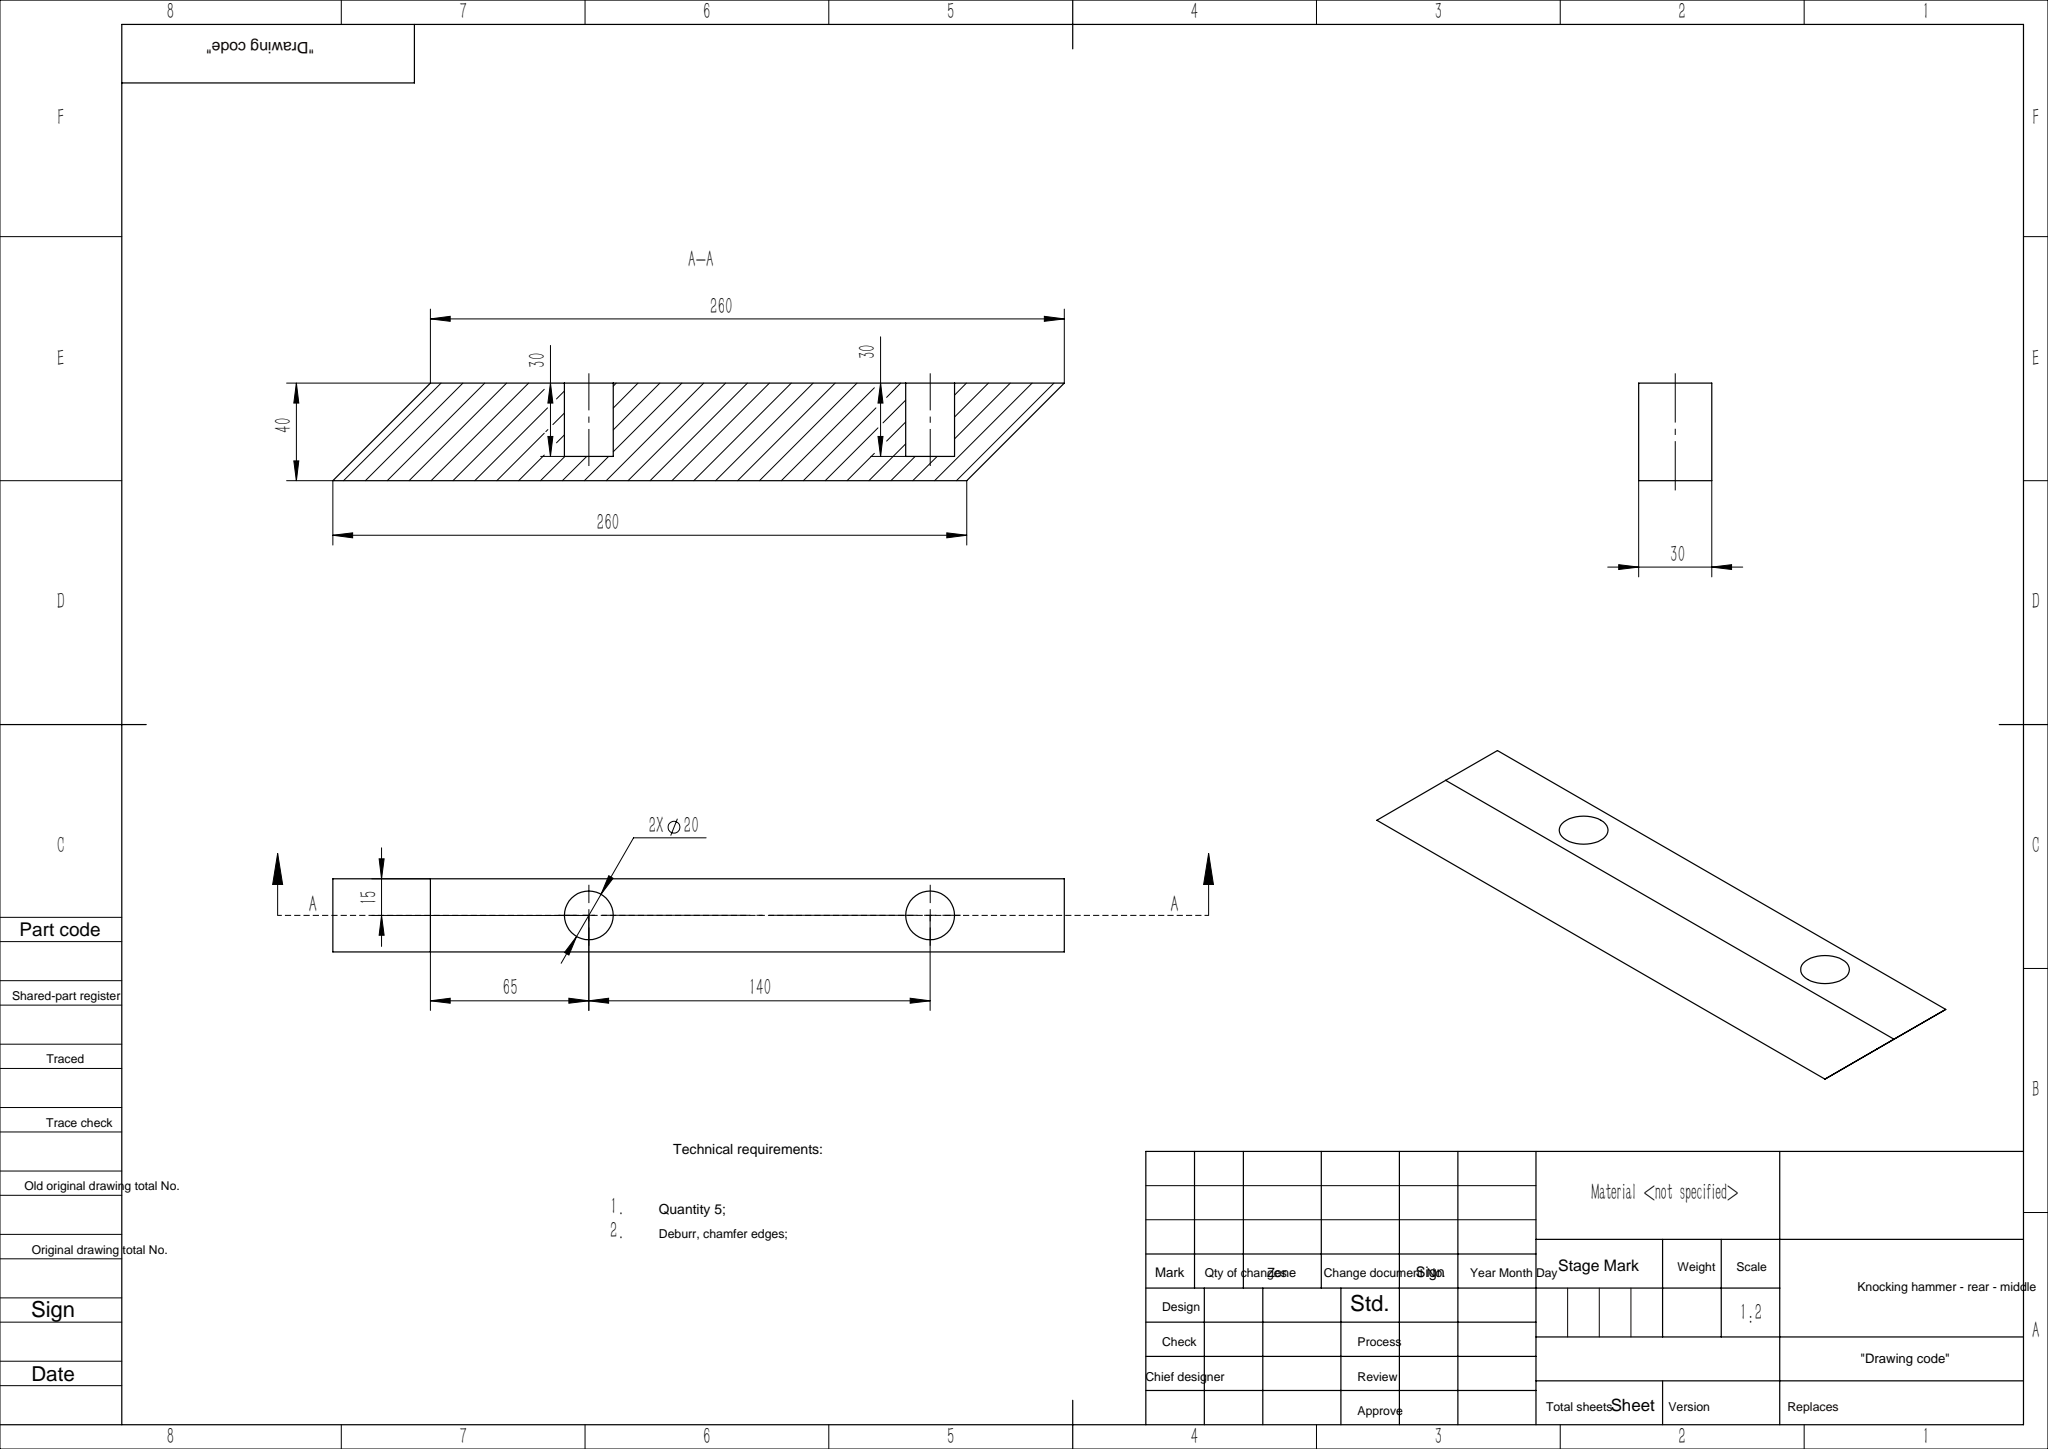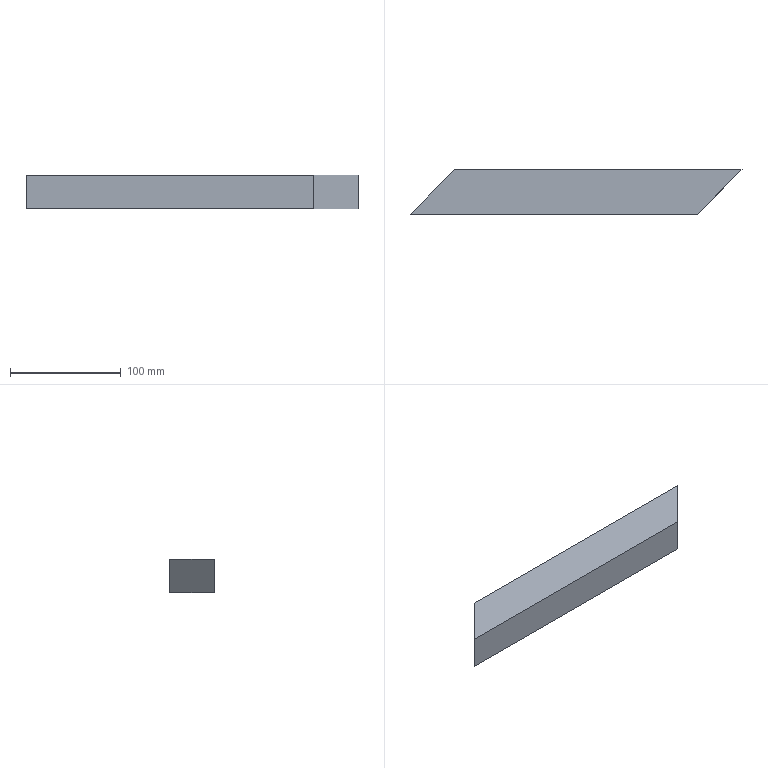Part | SolidWorks | features ICE 5, Extrusion 1 | 1 solid | 12 faces | box 300 x 40 x 30 mm | volume 293150 mm3 | plane 8 | cylinder 4 | commonest cylinder face diameters 20 x4
STEP:
#1=CARTESIAN_POINT('',(-70.,10.,-10.));
#2=VERTEX_POINT('',#1);
#3=CARTESIAN_POINT('',(-70.,10.,10.));
#4=VERTEX_POINT('',#3);
#5=CARTESIAN_POINT('',(-70.,10.,0.));
#6=DIRECTION('',(0.,1.,0.));
#7=DIRECTION('',(0.,0.,-1.));
#8=AXIS2_PLACEMENT_3D('',#5,#6,#7);
#9=CIRCLE('',#8,10.);
#10=EDGE_CURVE('',#2,#4,#9,.T.);
#11=ORIENTED_EDGE('',*,*,#10,.F.);
#12=CARTESIAN_POINT('',(-70.,40.,-10.));
#13=VERTEX_POINT('',#12);
#14=CARTESIAN_POINT('',(-70.,10.,-10.));
#15=DIRECTION('',(0.,1.,0.));
#16=VECTOR('',#15,1000.);
#17=LINE('',#14,#16);
#18=EDGE_CURVE('',#2,#13,#17,.T.);
#19=ORIENTED_EDGE('',*,*,#18,.T.);
#20=CARTESIAN_POINT('',(-70.,40.,10.));
#21=VERTEX_POINT('',#20);
#22=CARTESIAN_POINT('',(-70.,40.,0.));
#23=DIRECTION('',(0.,1.,0.));
#24=DIRECTION('',(0.,0.,-1.));
#25=AXIS2_PLACEMENT_3D('',#22,#23,#24);
#26=CIRCLE('',#25,10.);
#27=EDGE_CURVE('',#13,#21,#26,.T.);
#28=ORIENTED_EDGE('',*,*,#27,.T.);
#29=CARTESIAN_POINT('',(-70.,10.,10.));
#30=DIRECTION('',(0.,1.,0.));
#31=VECTOR('',#30,1000.);
#32=LINE('',#29,#31);
#33=EDGE_CURVE('',#4,#21,#32,.T.);
#34=ORIENTED_EDGE('',*,*,#33,.F.);
#35=EDGE_LOOP('',(#11,#19,#28,#34));
#36=FACE_OUTER_BOUND('',#35,.T.);
#37=CARTESIAN_POINT('',(-70.,10.,0.));
#38=DIRECTION('',(0.,1.,0.));
#39=DIRECTION('',(0.,0.,1.));
#40=AXIS2_PLACEMENT_3D('',#37,#38,#39);
#41=CYLINDRICAL_SURFACE('',#40,10.);
#42=ADVANCED_FACE('',(#36),#41,.F.);
#43=CARTESIAN_POINT('',(70.,10.,-10.));
#44=VERTEX_POINT('',#43);
#45=CARTESIAN_POINT('',(70.,10.,10.));
#46=VERTEX_POINT('',#45);
#47=CARTESIAN_POINT('',(70.,10.,0.));
#48=DIRECTION('',(0.,1.,0.));
#49=DIRECTION('',(0.,0.,1.));
#50=AXIS2_PLACEMENT_3D('',#47,#48,#49);
#51=CIRCLE('',#50,10.);
#52=EDGE_CURVE('',#44,#46,#51,.T.);
#53=ORIENTED_EDGE('',*,*,#52,.F.);
#54=CARTESIAN_POINT('',(70.,40.,-10.));
#55=VERTEX_POINT('',#54);
#56=CARTESIAN_POINT('',(70.,10.,-10.));
#57=DIRECTION('',(0.,1.,0.));
#58=VECTOR('',#57,1000.);
#59=LINE('',#56,#58);
#60=EDGE_CURVE('',#44,#55,#59,.T.);
#61=ORIENTED_EDGE('',*,*,#60,.T.);
#62=CARTESIAN_POINT('',(70.,40.,10.));
#63=VERTEX_POINT('',#62);
#64=CARTESIAN_POINT('',(70.,40.,0.));
#65=DIRECTION('',(0.,1.,0.));
#66=DIRECTION('',(0.,0.,1.));
#67=AXIS2_PLACEMENT_3D('',#64,#65,#66);
#68=CIRCLE('',#67,10.);
#69=EDGE_CURVE('',#55,#63,#68,.T.);
#70=ORIENTED_EDGE('',*,*,#69,.T.);
#71=CARTESIAN_POINT('',(70.,10.,10.));
#72=DIRECTION('',(0.,1.,0.));
#73=VECTOR('',#72,1000.);
#74=LINE('',#71,#73);
#75=EDGE_CURVE('',#46,#63,#74,.T.);
#76=ORIENTED_EDGE('',*,*,#75,.F.);
#77=EDGE_LOOP('',(#53,#61,#70,#76));
#78=FACE_OUTER_BOUND('',#77,.T.);
#79=CARTESIAN_POINT('',(70.,10.,0.));
#80=DIRECTION('',(0.,1.,0.));
#81=DIRECTION('',(0.,0.,1.));
#82=AXIS2_PLACEMENT_3D('',#79,#80,#81);
#83=CYLINDRICAL_SURFACE('',#82,10.);
#84=ADVANCED_FACE('',(#78),#83,.F.);
#85=CARTESIAN_POINT('',(85.,0.,-15.));
#86=VERTEX_POINT('',#85);
#87=CARTESIAN_POINT('',(-175.,0.,-15.));
#88=VERTEX_POINT('',#87);
#89=CARTESIAN_POINT('',(-135.,0.,-15.));
#90=DIRECTION('',(-1.,0.,0.));
#91=VECTOR('',#90,1000.);
#92=LINE('',#89,#91);
#93=EDGE_CURVE('',#86,#88,#92,.T.);
#94=ORIENTED_EDGE('',*,*,#93,.T.);
#95=CARTESIAN_POINT('',(-135.,40.,-15.));
#96=VERTEX_POINT('',#95);
#97=CARTESIAN_POINT('',(-175.,0.,-15.));
#98=DIRECTION('',(0.7071,0.7071,0.));
#99=VECTOR('',#98,1000.);
#100=LINE('',#97,#99);
#101=EDGE_CURVE('',#88,#96,#100,.T.);
#102=ORIENTED_EDGE('',*,*,#101,.T.);
#103=CARTESIAN_POINT('',(125.,40.,-15.));
#104=VERTEX_POINT('',#103);
#105=CARTESIAN_POINT('',(-135.,40.,-15.));
#106=DIRECTION('',(-1.,0.,0.));
#107=VECTOR('',#106,1000.);
#108=LINE('',#105,#107);
#109=EDGE_CURVE('',#104,#96,#108,.T.);
#110=ORIENTED_EDGE('',*,*,#109,.F.);
#111=CARTESIAN_POINT('',(125.,40.,-15.));
#112=DIRECTION('',(-0.7071,-0.7071,0.));
#113=VECTOR('',#112,1000.);
#114=LINE('',#111,#113);
#115=EDGE_CURVE('',#104,#86,#114,.T.);
#116=ORIENTED_EDGE('',*,*,#115,.T.);
#117=EDGE_LOOP('',(#94,#102,#110,#116));
#118=FACE_OUTER_BOUND('',#117,.T.);
#119=CARTESIAN_POINT('',(-135.,40.,-15.));
#120=DIRECTION('',(0.,0.,1.));
#121=DIRECTION('',(1.,0.,0.));
#122=AXIS2_PLACEMENT_3D('',#119,#120,#121);
#123=PLANE('',#122);
#124=ADVANCED_FACE('',(#118),#123,.F.);
#125=CARTESIAN_POINT('',(-135.,40.,15.));
#126=VERTEX_POINT('',#125);
#127=CARTESIAN_POINT('',(125.,40.,15.));
#128=VERTEX_POINT('',#127);
#129=CARTESIAN_POINT('',(-135.,40.,15.));
#130=DIRECTION('',(1.,0.,0.));
#131=VECTOR('',#130,1000.);
#132=LINE('',#129,#131);
#133=EDGE_CURVE('',#126,#128,#132,.T.);
#134=ORIENTED_EDGE('',*,*,#133,.F.);
#135=CARTESIAN_POINT('',(-175.,0.,15.));
#136=VERTEX_POINT('',#135);
#137=CARTESIAN_POINT('',(-175.,0.,15.));
#138=DIRECTION('',(0.7071,0.7071,0.));
#139=VECTOR('',#138,1000.);
#140=LINE('',#137,#139);
#141=EDGE_CURVE('',#136,#126,#140,.T.);
#142=ORIENTED_EDGE('',*,*,#141,.F.);
#143=CARTESIAN_POINT('',(85.,0.,15.));
#144=VERTEX_POINT('',#143);
#145=CARTESIAN_POINT('',(-135.,0.,15.));
#146=DIRECTION('',(1.,0.,0.));
#147=VECTOR('',#146,1000.);
#148=LINE('',#145,#147);
#149=EDGE_CURVE('',#136,#144,#148,.T.);
#150=ORIENTED_EDGE('',*,*,#149,.T.);
#151=CARTESIAN_POINT('',(125.,40.,15.));
#152=DIRECTION('',(-0.7071,-0.7071,0.));
#153=VECTOR('',#152,1000.);
#154=LINE('',#151,#153);
#155=EDGE_CURVE('',#128,#144,#154,.T.);
#156=ORIENTED_EDGE('',*,*,#155,.F.);
#157=EDGE_LOOP('',(#134,#142,#150,#156));
#158=FACE_OUTER_BOUND('',#157,.T.);
#159=CARTESIAN_POINT('',(-135.,40.,15.));
#160=DIRECTION('',(0.,0.,-1.));
#161=DIRECTION('',(-1.,0.,0.));
#162=AXIS2_PLACEMENT_3D('',#159,#160,#161);
#163=PLANE('',#162);
#164=ADVANCED_FACE('',(#158),#163,.F.);
#165=CARTESIAN_POINT('',(70.,40.,0.));
#166=DIRECTION('',(0.,1.,0.));
#167=DIRECTION('',(0.,0.,1.));
#168=AXIS2_PLACEMENT_3D('',#165,#166,#167);
#169=CIRCLE('',#168,10.);
#170=EDGE_CURVE('',#63,#55,#169,.T.);
#171=ORIENTED_EDGE('',*,*,#170,.F.);
#172=ORIENTED_EDGE('',*,*,#69,.F.);
#173=EDGE_LOOP('',(#171,#172));
#174=FACE_BOUND('',#173,.T.);
#175=CARTESIAN_POINT('',(-70.,40.,0.));
#176=DIRECTION('',(0.,1.,0.));
#177=DIRECTION('',(0.,0.,-1.));
#178=AXIS2_PLACEMENT_3D('',#175,#176,#177);
#179=CIRCLE('',#178,10.);
#180=EDGE_CURVE('',#21,#13,#179,.T.);
#181=ORIENTED_EDGE('',*,*,#180,.F.);
#182=ORIENTED_EDGE('',*,*,#27,.F.);
#183=EDGE_LOOP('',(#181,#182));
#184=FACE_BOUND('',#183,.T.);
#185=ORIENTED_EDGE('',*,*,#109,.T.);
#186=CARTESIAN_POINT('',(-135.,40.,-15.));
#187=DIRECTION('',(0.,0.,1.));
#188=VECTOR('',#187,1000.);
#189=LINE('',#186,#188);
#190=EDGE_CURVE('',#96,#126,#189,.T.);
#191=ORIENTED_EDGE('',*,*,#190,.T.);
#192=ORIENTED_EDGE('',*,*,#133,.T.);
#193=CARTESIAN_POINT('',(125.,40.,-15.));
#194=DIRECTION('',(0.,0.,1.));
#195=VECTOR('',#194,1000.);
#196=LINE('',#193,#195);
#197=EDGE_CURVE('',#104,#128,#196,.T.);
#198=ORIENTED_EDGE('',*,*,#197,.F.);
#199=EDGE_LOOP('',(#185,#191,#192,#198));
#200=FACE_OUTER_BOUND('',#199,.T.);
#201=CARTESIAN_POINT('',(0.,40.,0.));
#202=DIRECTION('',(0.,-1.,0.));
#203=DIRECTION('',(0.,0.,-1.));
#204=AXIS2_PLACEMENT_3D('',#201,#202,#203);
#205=PLANE('',#204);
#206=ADVANCED_FACE('',(#174,#184,#200),#205,.F.);
#207=CARTESIAN_POINT('',(85.,0.,-15.));
#208=DIRECTION('',(0.,0.,1.));
#209=VECTOR('',#208,1000.);
#210=LINE('',#207,#209);
#211=EDGE_CURVE('',#86,#144,#210,.T.);
#212=ORIENTED_EDGE('',*,*,#211,.T.);
#213=ORIENTED_EDGE('',*,*,#149,.F.);
#214=CARTESIAN_POINT('',(-175.,0.,-15.));
#215=DIRECTION('',(0.,0.,1.));
#216=VECTOR('',#215,1000.);
#217=LINE('',#214,#216);
#218=EDGE_CURVE('',#88,#136,#217,.T.);
#219=ORIENTED_EDGE('',*,*,#218,.F.);
#220=ORIENTED_EDGE('',*,*,#93,.F.);
#221=EDGE_LOOP('',(#212,#213,#219,#220));
#222=FACE_OUTER_BOUND('',#221,.T.);
#223=CARTESIAN_POINT('',(0.,0.,0.));
#224=DIRECTION('',(0.,-1.,0.));
#225=DIRECTION('',(0.,0.,-1.));
#226=AXIS2_PLACEMENT_3D('',#223,#224,#225);
#227=PLANE('',#226);
#228=ADVANCED_FACE('',(#222),#227,.T.);
#229=ORIENTED_EDGE('',*,*,#60,.F.);
#230=CARTESIAN_POINT('',(70.,10.,0.));
#231=DIRECTION('',(0.,1.,0.));
#232=DIRECTION('',(0.,0.,1.));
#233=AXIS2_PLACEMENT_3D('',#230,#231,#232);
#234=CIRCLE('',#233,10.);
#235=EDGE_CURVE('',#46,#44,#234,.T.);
#236=ORIENTED_EDGE('',*,*,#235,.F.);
#237=ORIENTED_EDGE('',*,*,#75,.T.);
#238=ORIENTED_EDGE('',*,*,#170,.T.);
#239=EDGE_LOOP('',(#229,#236,#237,#238));
#240=FACE_OUTER_BOUND('',#239,.T.);
#241=CARTESIAN_POINT('',(70.,10.,0.));
#242=DIRECTION('',(0.,1.,0.));
#243=DIRECTION('',(0.,0.,1.));
#244=AXIS2_PLACEMENT_3D('',#241,#242,#243);
#245=CYLINDRICAL_SURFACE('',#244,10.);
#246=ADVANCED_FACE('',(#240),#245,.F.);
#247=ORIENTED_EDGE('',*,*,#235,.T.);
#248=ORIENTED_EDGE('',*,*,#52,.T.);
#249=EDGE_LOOP('',(#247,#248));
#250=FACE_OUTER_BOUND('',#249,.T.);
#251=CARTESIAN_POINT('',(70.,10.,0.));
#252=DIRECTION('',(0.,1.,0.));
#253=DIRECTION('',(0.,0.,1.));
#254=AXIS2_PLACEMENT_3D('',#251,#252,#253);
#255=PLANE('',#254);
#256=ADVANCED_FACE('',(#250),#255,.T.);
#257=ORIENTED_EDGE('',*,*,#18,.F.);
#258=CARTESIAN_POINT('',(-70.,10.,0.));
#259=DIRECTION('',(0.,1.,0.));
#260=DIRECTION('',(0.,0.,-1.));
#261=AXIS2_PLACEMENT_3D('',#258,#259,#260);
#262=CIRCLE('',#261,10.);
#263=EDGE_CURVE('',#4,#2,#262,.T.);
#264=ORIENTED_EDGE('',*,*,#263,.F.);
#265=ORIENTED_EDGE('',*,*,#33,.T.);
#266=ORIENTED_EDGE('',*,*,#180,.T.);
#267=EDGE_LOOP('',(#257,#264,#265,#266));
#268=FACE_OUTER_BOUND('',#267,.T.);
#269=CARTESIAN_POINT('',(-70.,10.,0.));
#270=DIRECTION('',(0.,1.,0.));
#271=DIRECTION('',(0.,0.,1.));
#272=AXIS2_PLACEMENT_3D('',#269,#270,#271);
#273=CYLINDRICAL_SURFACE('',#272,10.);
#274=ADVANCED_FACE('',(#268),#273,.F.);
#275=ORIENTED_EDGE('',*,*,#263,.T.);
#276=ORIENTED_EDGE('',*,*,#10,.T.);
#277=EDGE_LOOP('',(#275,#276));
#278=FACE_OUTER_BOUND('',#277,.T.);
#279=CARTESIAN_POINT('',(-70.,10.,0.));
#280=DIRECTION('',(0.,-1.,0.));
#281=DIRECTION('',(0.,0.,-1.));
#282=AXIS2_PLACEMENT_3D('',#279,#280,#281);
#283=PLANE('',#282);
#284=ADVANCED_FACE('',(#278),#283,.F.);
#285=ORIENTED_EDGE('',*,*,#155,.T.);
#286=ORIENTED_EDGE('',*,*,#211,.F.);
#287=ORIENTED_EDGE('',*,*,#115,.F.);
#288=ORIENTED_EDGE('',*,*,#197,.T.);
#289=EDGE_LOOP('',(#285,#286,#287,#288));
#290=FACE_OUTER_BOUND('',#289,.T.);
#291=CARTESIAN_POINT('',(125.,40.,-15.));
#292=DIRECTION('',(-0.7071,0.7071,0.));
#293=DIRECTION('',(-0.7071,-0.7071,0.));
#294=AXIS2_PLACEMENT_3D('',#291,#292,#293);
#295=PLANE('',#294);
#296=ADVANCED_FACE('',(#290),#295,.F.);
#297=ORIENTED_EDGE('',*,*,#141,.T.);
#298=ORIENTED_EDGE('',*,*,#190,.F.);
#299=ORIENTED_EDGE('',*,*,#101,.F.);
#300=ORIENTED_EDGE('',*,*,#218,.T.);
#301=EDGE_LOOP('',(#297,#298,#299,#300));
#302=FACE_OUTER_BOUND('',#301,.T.);
#303=CARTESIAN_POINT('',(-175.,0.,-15.));
#304=DIRECTION('',(0.7071,-0.7071,0.));
#305=DIRECTION('',(0.7071,0.7071,0.));
#306=AXIS2_PLACEMENT_3D('',#303,#304,#305);
#307=PLANE('',#306);
#308=ADVANCED_FACE('',(#302),#307,.F.);
#309=CLOSED_SHELL('',(#42,#84,#124,#164,#206,#228,#246,#256,#274,#284,#296,#308));
#310=MANIFOLD_SOLID_BREP('',#309);
#311=CARTESIAN_POINT('',(0.,0.,0.));
#312=DIRECTION('',(0.,0.,1.));
#313=DIRECTION('',(1.,0.,0.));
#314=AXIS2_PLACEMENT_3D('',#311,#312,#313);
#315=(LENGTH_UNIT()NAMED_UNIT(*)SI_UNIT(.MILLI.,.METRE.));
#316=UNCERTAINTY_MEASURE_WITH_UNIT(LENGTH_MEASURE(0.00001),#315,'','');
#317=(NAMED_UNIT(*)PLANE_ANGLE_UNIT()SI_UNIT($,.RADIAN.));
#318=(NAMED_UNIT(*)SI_UNIT($,.STERADIAN.)SOLID_ANGLE_UNIT());
#319=(GEOMETRIC_REPRESENTATION_CONTEXT(3)GLOBAL_UNCERTAINTY_ASSIGNED_CONTEXT((#316))GLOBAL_UNIT_ASSIGNED_CONTEXT((#315,#317,#318))REPRESENTATION_CONTEXT('',''));
#320=ADVANCED_BREP_SHAPE_REPRESENTATION('',(#310,#314),#319);